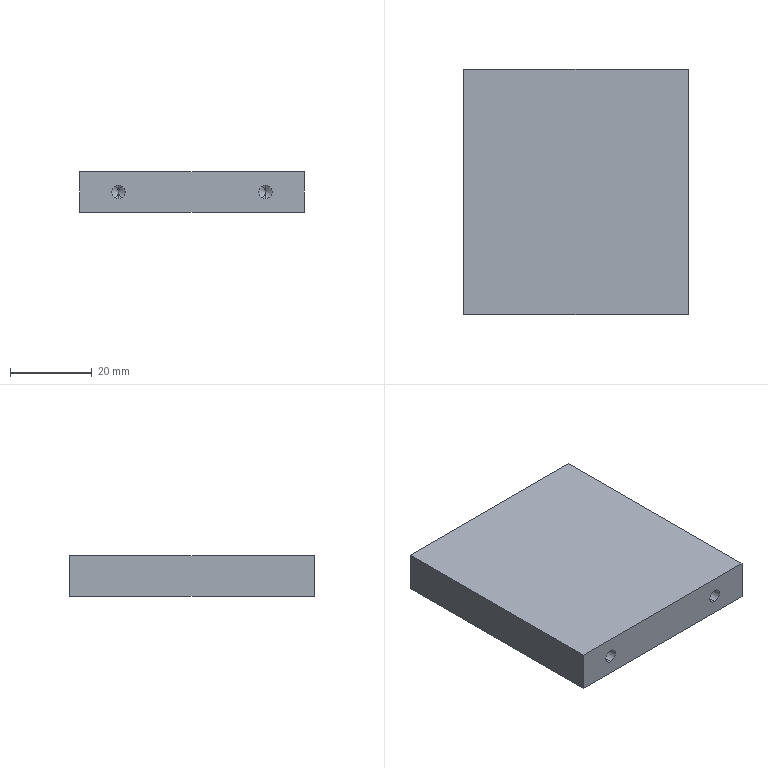Part | SolidWorks | features Extrusion 1, HoleWzd 1, MirrorPattern 1 | 1 solid | 22 faces | box 55 x 60 x 10 mm | volume 32595 mm3 | cylinder 8 | cone 8 | plane 6 | commonest cylinder face diameters 3.3 x8
STEP:
#1=CARTESIAN_POINT('',(18.,18.5,-1.65));
#2=VERTEX_POINT('',#1);
#3=CARTESIAN_POINT('',(18.,18.5,1.65));
#4=VERTEX_POINT('',#3);
#5=CARTESIAN_POINT('',(18.,18.5,0.));
#6=DIRECTION('',(0.,1.,0.));
#7=DIRECTION('',(0.,0.,1.));
#8=AXIS2_PLACEMENT_3D('',#5,#6,#7);
#9=CIRCLE('',#8,1.65);
#10=EDGE_CURVE('',#2,#4,#9,.T.);
#11=ORIENTED_EDGE('',*,*,#10,.F.);
#12=CARTESIAN_POINT('',(18.,30.,-1.65));
#13=VERTEX_POINT('',#12);
#14=CARTESIAN_POINT('',(18.,30.,-1.65));
#15=DIRECTION('',(0.,1.,0.));
#16=VECTOR('',#15,1000.);
#17=LINE('',#14,#16);
#18=EDGE_CURVE('',#2,#13,#17,.T.);
#19=ORIENTED_EDGE('',*,*,#18,.T.);
#20=CARTESIAN_POINT('',(18.,30.,1.65));
#21=VERTEX_POINT('',#20);
#22=CARTESIAN_POINT('',(18.,30.,0.));
#23=DIRECTION('',(0.,1.,0.));
#24=DIRECTION('',(0.,0.,1.));
#25=AXIS2_PLACEMENT_3D('',#22,#23,#24);
#26=CIRCLE('',#25,1.65);
#27=EDGE_CURVE('',#13,#21,#26,.T.);
#28=ORIENTED_EDGE('',*,*,#27,.T.);
#29=CARTESIAN_POINT('',(18.,30.,1.65));
#30=DIRECTION('',(0.,1.,0.));
#31=VECTOR('',#30,1000.);
#32=LINE('',#29,#31);
#33=EDGE_CURVE('',#4,#21,#32,.T.);
#34=ORIENTED_EDGE('',*,*,#33,.F.);
#35=EDGE_LOOP('',(#11,#19,#28,#34));
#36=FACE_OUTER_BOUND('',#35,.T.);
#37=CARTESIAN_POINT('',(18.,30.,0.));
#38=DIRECTION('',(0.,1.,0.));
#39=DIRECTION('',(0.,0.,1.));
#40=AXIS2_PLACEMENT_3D('',#37,#38,#39);
#41=CYLINDRICAL_SURFACE('',#40,1.65);
#42=ADVANCED_FACE('',(#36),#41,.F.);
#43=CARTESIAN_POINT('',(18.,17.509,0.));
#44=VERTEX_POINT('',#43);
#45=CARTESIAN_POINT('',(18.,18.5,1.65));
#46=DIRECTION('',(0.,0.515,0.8572));
#47=VECTOR('',#46,1000.);
#48=LINE('',#45,#47);
#49=EDGE_CURVE('',#44,#4,#48,.T.);
#50=ORIENTED_EDGE('',*,*,#49,.F.);
#51=CARTESIAN_POINT('',(18.,18.5,-1.65));
#52=DIRECTION('',(0.,0.515,-0.8572));
#53=VECTOR('',#52,1000.);
#54=LINE('',#51,#53);
#55=EDGE_CURVE('',#44,#2,#54,.T.);
#56=ORIENTED_EDGE('',*,*,#55,.T.);
#57=ORIENTED_EDGE('',*,*,#10,.T.);
#58=EDGE_LOOP('',(#50,#56,#57));
#59=FACE_OUTER_BOUND('',#58,.T.);
#60=CARTESIAN_POINT('',(18.,18.5,0.));
#61=DIRECTION('',(0.,1.,0.));
#62=DIRECTION('',(0.,0.,1.));
#63=AXIS2_PLACEMENT_3D('',#60,#61,#62);
#64=CONICAL_SURFACE('',#63,1.65,1.03);
#65=ADVANCED_FACE('',(#59),#64,.F.);
#66=CARTESIAN_POINT('',(-18.,18.5,-1.65));
#67=VERTEX_POINT('',#66);
#68=CARTESIAN_POINT('',(-18.,18.5,1.65));
#69=VERTEX_POINT('',#68);
#70=CARTESIAN_POINT('',(-18.,18.5,0.));
#71=DIRECTION('',(0.,1.,0.));
#72=DIRECTION('',(0.,0.,1.));
#73=AXIS2_PLACEMENT_3D('',#70,#71,#72);
#74=CIRCLE('',#73,1.65);
#75=EDGE_CURVE('',#67,#69,#74,.T.);
#76=ORIENTED_EDGE('',*,*,#75,.F.);
#77=CARTESIAN_POINT('',(-18.,30.,-1.65));
#78=VERTEX_POINT('',#77);
#79=CARTESIAN_POINT('',(-18.,30.,-1.65));
#80=DIRECTION('',(0.,1.,0.));
#81=VECTOR('',#80,1000.);
#82=LINE('',#79,#81);
#83=EDGE_CURVE('',#67,#78,#82,.T.);
#84=ORIENTED_EDGE('',*,*,#83,.T.);
#85=CARTESIAN_POINT('',(-18.,30.,1.65));
#86=VERTEX_POINT('',#85);
#87=CARTESIAN_POINT('',(-18.,30.,0.));
#88=DIRECTION('',(0.,1.,0.));
#89=DIRECTION('',(0.,0.,1.));
#90=AXIS2_PLACEMENT_3D('',#87,#88,#89);
#91=CIRCLE('',#90,1.65);
#92=EDGE_CURVE('',#78,#86,#91,.T.);
#93=ORIENTED_EDGE('',*,*,#92,.T.);
#94=CARTESIAN_POINT('',(-18.,30.,1.65));
#95=DIRECTION('',(0.,1.,0.));
#96=VECTOR('',#95,1000.);
#97=LINE('',#94,#96);
#98=EDGE_CURVE('',#69,#86,#97,.T.);
#99=ORIENTED_EDGE('',*,*,#98,.F.);
#100=EDGE_LOOP('',(#76,#84,#93,#99));
#101=FACE_OUTER_BOUND('',#100,.T.);
#102=CARTESIAN_POINT('',(-18.,30.,0.));
#103=DIRECTION('',(0.,1.,0.));
#104=DIRECTION('',(0.,0.,1.));
#105=AXIS2_PLACEMENT_3D('',#102,#103,#104);
#106=CYLINDRICAL_SURFACE('',#105,1.65);
#107=ADVANCED_FACE('',(#101),#106,.F.);
#108=CARTESIAN_POINT('',(-18.,17.509,0.));
#109=VERTEX_POINT('',#108);
#110=CARTESIAN_POINT('',(-18.,18.5,1.65));
#111=DIRECTION('',(0.,0.515,0.8572));
#112=VECTOR('',#111,1000.);
#113=LINE('',#110,#112);
#114=EDGE_CURVE('',#109,#69,#113,.T.);
#115=ORIENTED_EDGE('',*,*,#114,.F.);
#116=CARTESIAN_POINT('',(-18.,18.5,-1.65));
#117=DIRECTION('',(0.,0.515,-0.8572));
#118=VECTOR('',#117,1000.);
#119=LINE('',#116,#118);
#120=EDGE_CURVE('',#109,#67,#119,.T.);
#121=ORIENTED_EDGE('',*,*,#120,.T.);
#122=ORIENTED_EDGE('',*,*,#75,.T.);
#123=EDGE_LOOP('',(#115,#121,#122));
#124=FACE_OUTER_BOUND('',#123,.T.);
#125=CARTESIAN_POINT('',(-18.,18.5,0.));
#126=DIRECTION('',(0.,1.,0.));
#127=DIRECTION('',(0.,0.,1.));
#128=AXIS2_PLACEMENT_3D('',#125,#126,#127);
#129=CONICAL_SURFACE('',#128,1.65,1.03);
#130=ADVANCED_FACE('',(#124),#129,.F.);
#131=CARTESIAN_POINT('',(18.,-18.5,1.65));
#132=VERTEX_POINT('',#131);
#133=CARTESIAN_POINT('',(18.,-18.5,-1.65));
#134=VERTEX_POINT('',#133);
#135=CARTESIAN_POINT('',(18.,-18.5,0.));
#136=DIRECTION('',(0.,-1.,0.));
#137=DIRECTION('',(0.,0.,-1.));
#138=AXIS2_PLACEMENT_3D('',#135,#136,#137);
#139=CIRCLE('',#138,1.65);
#140=EDGE_CURVE('',#132,#134,#139,.T.);
#141=ORIENTED_EDGE('',*,*,#140,.F.);
#142=CARTESIAN_POINT('',(18.,-30.,1.65));
#143=VERTEX_POINT('',#142);
#144=CARTESIAN_POINT('',(18.,-30.,1.65));
#145=DIRECTION('',(0.,-1.,0.));
#146=VECTOR('',#145,1000.);
#147=LINE('',#144,#146);
#148=EDGE_CURVE('',#132,#143,#147,.T.);
#149=ORIENTED_EDGE('',*,*,#148,.T.);
#150=CARTESIAN_POINT('',(18.,-30.,-1.65));
#151=VERTEX_POINT('',#150);
#152=CARTESIAN_POINT('',(18.,-30.,0.));
#153=DIRECTION('',(0.,-1.,0.));
#154=DIRECTION('',(0.,0.,-1.));
#155=AXIS2_PLACEMENT_3D('',#152,#153,#154);
#156=CIRCLE('',#155,1.65);
#157=EDGE_CURVE('',#143,#151,#156,.T.);
#158=ORIENTED_EDGE('',*,*,#157,.T.);
#159=CARTESIAN_POINT('',(18.,-30.,-1.65));
#160=DIRECTION('',(0.,-1.,0.));
#161=VECTOR('',#160,1000.);
#162=LINE('',#159,#161);
#163=EDGE_CURVE('',#134,#151,#162,.T.);
#164=ORIENTED_EDGE('',*,*,#163,.F.);
#165=EDGE_LOOP('',(#141,#149,#158,#164));
#166=FACE_OUTER_BOUND('',#165,.T.);
#167=CARTESIAN_POINT('',(18.,-30.,0.));
#168=DIRECTION('',(0.,-1.,0.));
#169=DIRECTION('',(0.,0.,-1.));
#170=AXIS2_PLACEMENT_3D('',#167,#168,#169);
#171=CYLINDRICAL_SURFACE('',#170,1.65);
#172=ADVANCED_FACE('',(#166),#171,.F.);
#173=CARTESIAN_POINT('',(18.,-17.509,0.));
#174=VERTEX_POINT('',#173);
#175=CARTESIAN_POINT('',(18.,-18.5,-1.65));
#176=DIRECTION('',(0.,-0.515,-0.8572));
#177=VECTOR('',#176,1000.);
#178=LINE('',#175,#177);
#179=EDGE_CURVE('',#174,#134,#178,.T.);
#180=ORIENTED_EDGE('',*,*,#179,.F.);
#181=CARTESIAN_POINT('',(18.,-18.5,1.65));
#182=DIRECTION('',(0.,-0.515,0.8572));
#183=VECTOR('',#182,1000.);
#184=LINE('',#181,#183);
#185=EDGE_CURVE('',#174,#132,#184,.T.);
#186=ORIENTED_EDGE('',*,*,#185,.T.);
#187=ORIENTED_EDGE('',*,*,#140,.T.);
#188=EDGE_LOOP('',(#180,#186,#187));
#189=FACE_OUTER_BOUND('',#188,.T.);
#190=CARTESIAN_POINT('',(18.,-18.5,0.));
#191=DIRECTION('',(0.,-1.,0.));
#192=DIRECTION('',(0.,0.,-1.));
#193=AXIS2_PLACEMENT_3D('',#190,#191,#192);
#194=CONICAL_SURFACE('',#193,1.65,1.03);
#195=ADVANCED_FACE('',(#189),#194,.F.);
#196=CARTESIAN_POINT('',(-18.,-18.5,1.65));
#197=VERTEX_POINT('',#196);
#198=CARTESIAN_POINT('',(-18.,-18.5,-1.65));
#199=VERTEX_POINT('',#198);
#200=CARTESIAN_POINT('',(-18.,-18.5,0.));
#201=DIRECTION('',(0.,-1.,0.));
#202=DIRECTION('',(0.,0.,-1.));
#203=AXIS2_PLACEMENT_3D('',#200,#201,#202);
#204=CIRCLE('',#203,1.65);
#205=EDGE_CURVE('',#197,#199,#204,.T.);
#206=ORIENTED_EDGE('',*,*,#205,.F.);
#207=CARTESIAN_POINT('',(-18.,-30.,1.65));
#208=VERTEX_POINT('',#207);
#209=CARTESIAN_POINT('',(-18.,-30.,1.65));
#210=DIRECTION('',(0.,-1.,0.));
#211=VECTOR('',#210,1000.);
#212=LINE('',#209,#211);
#213=EDGE_CURVE('',#197,#208,#212,.T.);
#214=ORIENTED_EDGE('',*,*,#213,.T.);
#215=CARTESIAN_POINT('',(-18.,-30.,-1.65));
#216=VERTEX_POINT('',#215);
#217=CARTESIAN_POINT('',(-18.,-30.,0.));
#218=DIRECTION('',(0.,-1.,0.));
#219=DIRECTION('',(0.,0.,-1.));
#220=AXIS2_PLACEMENT_3D('',#217,#218,#219);
#221=CIRCLE('',#220,1.65);
#222=EDGE_CURVE('',#208,#216,#221,.T.);
#223=ORIENTED_EDGE('',*,*,#222,.T.);
#224=CARTESIAN_POINT('',(-18.,-30.,-1.65));
#225=DIRECTION('',(0.,-1.,0.));
#226=VECTOR('',#225,1000.);
#227=LINE('',#224,#226);
#228=EDGE_CURVE('',#199,#216,#227,.T.);
#229=ORIENTED_EDGE('',*,*,#228,.F.);
#230=EDGE_LOOP('',(#206,#214,#223,#229));
#231=FACE_OUTER_BOUND('',#230,.T.);
#232=CARTESIAN_POINT('',(-18.,-30.,0.));
#233=DIRECTION('',(0.,-1.,0.));
#234=DIRECTION('',(0.,0.,-1.));
#235=AXIS2_PLACEMENT_3D('',#232,#233,#234);
#236=CYLINDRICAL_SURFACE('',#235,1.65);
#237=ADVANCED_FACE('',(#231),#236,.F.);
#238=CARTESIAN_POINT('',(-18.,-17.509,0.));
#239=VERTEX_POINT('',#238);
#240=CARTESIAN_POINT('',(-18.,-18.5,-1.65));
#241=DIRECTION('',(0.,-0.515,-0.8572));
#242=VECTOR('',#241,1000.);
#243=LINE('',#240,#242);
#244=EDGE_CURVE('',#239,#199,#243,.T.);
#245=ORIENTED_EDGE('',*,*,#244,.F.);
#246=CARTESIAN_POINT('',(-18.,-18.5,1.65));
#247=DIRECTION('',(0.,-0.515,0.8572));
#248=VECTOR('',#247,1000.);
#249=LINE('',#246,#248);
#250=EDGE_CURVE('',#239,#197,#249,.T.);
#251=ORIENTED_EDGE('',*,*,#250,.T.);
#252=ORIENTED_EDGE('',*,*,#205,.T.);
#253=EDGE_LOOP('',(#245,#251,#252));
#254=FACE_OUTER_BOUND('',#253,.T.);
#255=CARTESIAN_POINT('',(-18.,-18.5,0.));
#256=DIRECTION('',(0.,-1.,0.));
#257=DIRECTION('',(0.,0.,-1.));
#258=AXIS2_PLACEMENT_3D('',#255,#256,#257);
#259=CONICAL_SURFACE('',#258,1.65,1.03);
#260=ADVANCED_FACE('',(#254),#259,.F.);
#261=CARTESIAN_POINT('',(27.5,-30.,-5.));
#262=VERTEX_POINT('',#261);
#263=CARTESIAN_POINT('',(27.5,30.,-5.));
#264=VERTEX_POINT('',#263);
#265=CARTESIAN_POINT('',(27.5,30.,-5.));
#266=DIRECTION('',(0.,1.,0.));
#267=VECTOR('',#266,1000.);
#268=LINE('',#265,#267);
#269=EDGE_CURVE('',#262,#264,#268,.T.);
#270=ORIENTED_EDGE('',*,*,#269,.T.);
#271=CARTESIAN_POINT('',(27.5,30.,5.));
#272=VERTEX_POINT('',#271);
#273=CARTESIAN_POINT('',(27.5,30.,5.));
#274=DIRECTION('',(0.,0.,-1.));
#275=VECTOR('',#274,1000.);
#276=LINE('',#273,#275);
#277=EDGE_CURVE('',#272,#264,#276,.T.);
#278=ORIENTED_EDGE('',*,*,#277,.F.);
#279=CARTESIAN_POINT('',(27.5,-30.,5.));
#280=VERTEX_POINT('',#279);
#281=CARTESIAN_POINT('',(27.5,30.,5.));
#282=DIRECTION('',(0.,1.,0.));
#283=VECTOR('',#282,1000.);
#284=LINE('',#281,#283);
#285=EDGE_CURVE('',#280,#272,#284,.T.);
#286=ORIENTED_EDGE('',*,*,#285,.F.);
#287=CARTESIAN_POINT('',(27.5,-30.,5.));
#288=DIRECTION('',(0.,0.,-1.));
#289=VECTOR('',#288,1000.);
#290=LINE('',#287,#289);
#291=EDGE_CURVE('',#280,#262,#290,.T.);
#292=ORIENTED_EDGE('',*,*,#291,.T.);
#293=EDGE_LOOP('',(#270,#278,#286,#292));
#294=FACE_OUTER_BOUND('',#293,.T.);
#295=CARTESIAN_POINT('',(27.5,30.,5.));
#296=DIRECTION('',(-1.,0.,0.));
#297=DIRECTION('',(0.,-1.,0.));
#298=AXIS2_PLACEMENT_3D('',#295,#296,#297);
#299=PLANE('',#298);
#300=ADVANCED_FACE('',(#294),#299,.F.);
#301=CARTESIAN_POINT('',(18.,30.,0.));
#302=DIRECTION('',(0.,1.,0.));
#303=DIRECTION('',(0.,0.,1.));
#304=AXIS2_PLACEMENT_3D('',#301,#302,#303);
#305=CIRCLE('',#304,1.65);
#306=EDGE_CURVE('',#21,#13,#305,.T.);
#307=ORIENTED_EDGE('',*,*,#306,.F.);
#308=ORIENTED_EDGE('',*,*,#27,.F.);
#309=EDGE_LOOP('',(#307,#308));
#310=FACE_BOUND('',#309,.T.);
#311=CARTESIAN_POINT('',(-18.,30.,0.));
#312=DIRECTION('',(0.,1.,0.));
#313=DIRECTION('',(0.,0.,1.));
#314=AXIS2_PLACEMENT_3D('',#311,#312,#313);
#315=CIRCLE('',#314,1.65);
#316=EDGE_CURVE('',#86,#78,#315,.T.);
#317=ORIENTED_EDGE('',*,*,#316,.F.);
#318=ORIENTED_EDGE('',*,*,#92,.F.);
#319=EDGE_LOOP('',(#317,#318));
#320=FACE_BOUND('',#319,.T.);
#321=CARTESIAN_POINT('',(-27.5,30.,-5.));
#322=VERTEX_POINT('',#321);
#323=CARTESIAN_POINT('',(-27.5,30.,-5.));
#324=DIRECTION('',(-1.,0.,0.));
#325=VECTOR('',#324,1000.);
#326=LINE('',#323,#325);
#327=EDGE_CURVE('',#264,#322,#326,.T.);
#328=ORIENTED_EDGE('',*,*,#327,.T.);
#329=CARTESIAN_POINT('',(-27.5,30.,5.));
#330=VERTEX_POINT('',#329);
#331=CARTESIAN_POINT('',(-27.5,30.,5.));
#332=DIRECTION('',(0.,0.,-1.));
#333=VECTOR('',#332,1000.);
#334=LINE('',#331,#333);
#335=EDGE_CURVE('',#330,#322,#334,.T.);
#336=ORIENTED_EDGE('',*,*,#335,.F.);
#337=CARTESIAN_POINT('',(-27.5,30.,5.));
#338=DIRECTION('',(-1.,0.,0.));
#339=VECTOR('',#338,1000.);
#340=LINE('',#337,#339);
#341=EDGE_CURVE('',#272,#330,#340,.T.);
#342=ORIENTED_EDGE('',*,*,#341,.F.);
#343=ORIENTED_EDGE('',*,*,#277,.T.);
#344=EDGE_LOOP('',(#328,#336,#342,#343));
#345=FACE_OUTER_BOUND('',#344,.T.);
#346=CARTESIAN_POINT('',(-27.5,30.,5.));
#347=DIRECTION('',(0.,-1.,0.));
#348=DIRECTION('',(0.,0.,-1.));
#349=AXIS2_PLACEMENT_3D('',#346,#347,#348);
#350=PLANE('',#349);
#351=ADVANCED_FACE('',(#310,#320,#345),#350,.F.);
#352=CARTESIAN_POINT('',(-27.5,-30.,-5.));
#353=VERTEX_POINT('',#352);
#354=CARTESIAN_POINT('',(-27.5,30.,-5.));
#355=DIRECTION('',(0.,-1.,0.));
#356=VECTOR('',#355,1000.);
#357=LINE('',#354,#356);
#358=EDGE_CURVE('',#322,#353,#357,.T.);
#359=ORIENTED_EDGE('',*,*,#358,.T.);
#360=CARTESIAN_POINT('',(-27.5,-30.,5.));
#361=VERTEX_POINT('',#360);
#362=CARTESIAN_POINT('',(-27.5,-30.,5.));
#363=DIRECTION('',(0.,0.,-1.));
#364=VECTOR('',#363,1000.);
#365=LINE('',#362,#364);
#366=EDGE_CURVE('',#361,#353,#365,.T.);
#367=ORIENTED_EDGE('',*,*,#366,.F.);
#368=CARTESIAN_POINT('',(-27.5,30.,5.));
#369=DIRECTION('',(0.,-1.,0.));
#370=VECTOR('',#369,1000.);
#371=LINE('',#368,#370);
#372=EDGE_CURVE('',#330,#361,#371,.T.);
#373=ORIENTED_EDGE('',*,*,#372,.F.);
#374=ORIENTED_EDGE('',*,*,#335,.T.);
#375=EDGE_LOOP('',(#359,#367,#373,#374));
#376=FACE_OUTER_BOUND('',#375,.T.);
#377=CARTESIAN_POINT('',(-27.5,30.,5.));
#378=DIRECTION('',(1.,0.,0.));
#379=DIRECTION('',(0.,1.,0.));
#380=AXIS2_PLACEMENT_3D('',#377,#378,#379);
#381=PLANE('',#380);
#382=ADVANCED_FACE('',(#376),#381,.F.);
#383=CARTESIAN_POINT('',(18.,-30.,0.));
#384=DIRECTION('',(0.,-1.,0.));
#385=DIRECTION('',(0.,0.,-1.));
#386=AXIS2_PLACEMENT_3D('',#383,#384,#385);
#387=CIRCLE('',#386,1.65);
#388=EDGE_CURVE('',#151,#143,#387,.T.);
#389=ORIENTED_EDGE('',*,*,#388,.F.);
#390=ORIENTED_EDGE('',*,*,#157,.F.);
#391=EDGE_LOOP('',(#389,#390));
#392=FACE_BOUND('',#391,.T.);
#393=CARTESIAN_POINT('',(-18.,-30.,0.));
#394=DIRECTION('',(0.,-1.,0.));
#395=DIRECTION('',(0.,0.,-1.));
#396=AXIS2_PLACEMENT_3D('',#393,#394,#395);
#397=CIRCLE('',#396,1.65);
#398=EDGE_CURVE('',#216,#208,#397,.T.);
#399=ORIENTED_EDGE('',*,*,#398,.F.);
#400=ORIENTED_EDGE('',*,*,#222,.F.);
#401=EDGE_LOOP('',(#399,#400));
#402=FACE_BOUND('',#401,.T.);
#403=CARTESIAN_POINT('',(-27.5,-30.,-5.));
#404=DIRECTION('',(1.,0.,0.));
#405=VECTOR('',#404,1000.);
#406=LINE('',#403,#405);
#407=EDGE_CURVE('',#353,#262,#406,.T.);
#408=ORIENTED_EDGE('',*,*,#407,.T.);
#409=ORIENTED_EDGE('',*,*,#291,.F.);
#410=CARTESIAN_POINT('',(-27.5,-30.,5.));
#411=DIRECTION('',(1.,0.,0.));
#412=VECTOR('',#411,1000.);
#413=LINE('',#410,#412);
#414=EDGE_CURVE('',#361,#280,#413,.T.);
#415=ORIENTED_EDGE('',*,*,#414,.F.);
#416=ORIENTED_EDGE('',*,*,#366,.T.);
#417=EDGE_LOOP('',(#408,#409,#415,#416));
#418=FACE_OUTER_BOUND('',#417,.T.);
#419=CARTESIAN_POINT('',(-27.5,-30.,5.));
#420=DIRECTION('',(0.,1.,0.));
#421=DIRECTION('',(0.,0.,1.));
#422=AXIS2_PLACEMENT_3D('',#419,#420,#421);
#423=PLANE('',#422);
#424=ADVANCED_FACE('',(#392,#402,#418),#423,.F.);
#425=ORIENTED_EDGE('',*,*,#285,.T.);
#426=ORIENTED_EDGE('',*,*,#341,.T.);
#427=ORIENTED_EDGE('',*,*,#372,.T.);
#428=ORIENTED_EDGE('',*,*,#414,.T.);
#429=EDGE_LOOP('',(#425,#426,#427,#428));
#430=FACE_OUTER_BOUND('',#429,.T.);
#431=CARTESIAN_POINT('',(0.,0.,5.));
#432=DIRECTION('',(0.,0.,1.));
#433=DIRECTION('',(1.,0.,0.));
#434=AXIS2_PLACEMENT_3D('',#431,#432,#433);
#435=PLANE('',#434);
#436=ADVANCED_FACE('',(#430),#435,.T.);
#437=ORIENTED_EDGE('',*,*,#269,.F.);
#438=ORIENTED_EDGE('',*,*,#407,.F.);
#439=ORIENTED_EDGE('',*,*,#358,.F.);
#440=ORIENTED_EDGE('',*,*,#327,.F.);
#441=EDGE_LOOP('',(#437,#438,#439,#440));
#442=FACE_OUTER_BOUND('',#441,.T.);
#443=CARTESIAN_POINT('',(0.,0.,-5.));
#444=DIRECTION('',(0.,0.,1.));
#445=DIRECTION('',(1.,0.,0.));
#446=AXIS2_PLACEMENT_3D('',#443,#444,#445);
#447=PLANE('',#446);
#448=ADVANCED_FACE('',(#442),#447,.F.);
#449=ORIENTED_EDGE('',*,*,#250,.F.);
#450=ORIENTED_EDGE('',*,*,#244,.T.);
#451=CARTESIAN_POINT('',(-18.,-18.5,0.));
#452=DIRECTION('',(0.,-1.,0.));
#453=DIRECTION('',(0.,0.,-1.));
#454=AXIS2_PLACEMENT_3D('',#451,#452,#453);
#455=CIRCLE('',#454,1.65);
#456=EDGE_CURVE('',#199,#197,#455,.T.);
#457=ORIENTED_EDGE('',*,*,#456,.T.);
#458=EDGE_LOOP('',(#449,#450,#457));
#459=FACE_OUTER_BOUND('',#458,.T.);
#460=CARTESIAN_POINT('',(-18.,-18.5,0.));
#461=DIRECTION('',(0.,-1.,0.));
#462=DIRECTION('',(0.,0.,-1.));
#463=AXIS2_PLACEMENT_3D('',#460,#461,#462);
#464=CONICAL_SURFACE('',#463,1.65,1.03);
#465=ADVANCED_FACE('',(#459),#464,.F.);
#466=ORIENTED_EDGE('',*,*,#213,.F.);
#467=ORIENTED_EDGE('',*,*,#456,.F.);
#468=ORIENTED_EDGE('',*,*,#228,.T.);
#469=ORIENTED_EDGE('',*,*,#398,.T.);
#470=EDGE_LOOP('',(#466,#467,#468,#469));
#471=FACE_OUTER_BOUND('',#470,.T.);
#472=CARTESIAN_POINT('',(-18.,-30.,0.));
#473=DIRECTION('',(0.,-1.,0.));
#474=DIRECTION('',(0.,0.,-1.));
#475=AXIS2_PLACEMENT_3D('',#472,#473,#474);
#476=CYLINDRICAL_SURFACE('',#475,1.65);
#477=ADVANCED_FACE('',(#471),#476,.F.);
#478=ORIENTED_EDGE('',*,*,#185,.F.);
#479=ORIENTED_EDGE('',*,*,#179,.T.);
#480=CARTESIAN_POINT('',(18.,-18.5,0.));
#481=DIRECTION('',(0.,-1.,0.));
#482=DIRECTION('',(0.,0.,-1.));
#483=AXIS2_PLACEMENT_3D('',#480,#481,#482);
#484=CIRCLE('',#483,1.65);
#485=EDGE_CURVE('',#134,#132,#484,.T.);
#486=ORIENTED_EDGE('',*,*,#485,.T.);
#487=EDGE_LOOP('',(#478,#479,#486));
#488=FACE_OUTER_BOUND('',#487,.T.);
#489=CARTESIAN_POINT('',(18.,-18.5,0.));
#490=DIRECTION('',(0.,-1.,0.));
#491=DIRECTION('',(0.,0.,-1.));
#492=AXIS2_PLACEMENT_3D('',#489,#490,#491);
#493=CONICAL_SURFACE('',#492,1.65,1.03);
#494=ADVANCED_FACE('',(#488),#493,.F.);
#495=ORIENTED_EDGE('',*,*,#148,.F.);
#496=ORIENTED_EDGE('',*,*,#485,.F.);
#497=ORIENTED_EDGE('',*,*,#163,.T.);
#498=ORIENTED_EDGE('',*,*,#388,.T.);
#499=EDGE_LOOP('',(#495,#496,#497,#498));
#500=FACE_OUTER_BOUND('',#499,.T.);
#501=CARTESIAN_POINT('',(18.,-30.,0.));
#502=DIRECTION('',(0.,-1.,0.));
#503=DIRECTION('',(0.,0.,-1.));
#504=AXIS2_PLACEMENT_3D('',#501,#502,#503);
#505=CYLINDRICAL_SURFACE('',#504,1.65);
#506=ADVANCED_FACE('',(#500),#505,.F.);
#507=ORIENTED_EDGE('',*,*,#120,.F.);
#508=ORIENTED_EDGE('',*,*,#114,.T.);
#509=CARTESIAN_POINT('',(-18.,18.5,0.));
#510=DIRECTION('',(0.,1.,0.));
#511=DIRECTION('',(0.,0.,1.));
#512=AXIS2_PLACEMENT_3D('',#509,#510,#511);
#513=CIRCLE('',#512,1.65);
#514=EDGE_CURVE('',#69,#67,#513,.T.);
#515=ORIENTED_EDGE('',*,*,#514,.T.);
#516=EDGE_LOOP('',(#507,#508,#515));
#517=FACE_OUTER_BOUND('',#516,.T.);
#518=CARTESIAN_POINT('',(-18.,18.5,0.));
#519=DIRECTION('',(0.,1.,0.));
#520=DIRECTION('',(0.,0.,1.));
#521=AXIS2_PLACEMENT_3D('',#518,#519,#520);
#522=CONICAL_SURFACE('',#521,1.65,1.03);
#523=ADVANCED_FACE('',(#517),#522,.F.);
#524=ORIENTED_EDGE('',*,*,#83,.F.);
#525=ORIENTED_EDGE('',*,*,#514,.F.);
#526=ORIENTED_EDGE('',*,*,#98,.T.);
#527=ORIENTED_EDGE('',*,*,#316,.T.);
#528=EDGE_LOOP('',(#524,#525,#526,#527));
#529=FACE_OUTER_BOUND('',#528,.T.);
#530=CARTESIAN_POINT('',(-18.,30.,0.));
#531=DIRECTION('',(0.,1.,0.));
#532=DIRECTION('',(0.,0.,1.));
#533=AXIS2_PLACEMENT_3D('',#530,#531,#532);
#534=CYLINDRICAL_SURFACE('',#533,1.65);
#535=ADVANCED_FACE('',(#529),#534,.F.);
#536=ORIENTED_EDGE('',*,*,#55,.F.);
#537=ORIENTED_EDGE('',*,*,#49,.T.);
#538=CARTESIAN_POINT('',(18.,18.5,0.));
#539=DIRECTION('',(0.,1.,0.));
#540=DIRECTION('',(0.,0.,1.));
#541=AXIS2_PLACEMENT_3D('',#538,#539,#540);
#542=CIRCLE('',#541,1.65);
#543=EDGE_CURVE('',#4,#2,#542,.T.);
#544=ORIENTED_EDGE('',*,*,#543,.T.);
#545=EDGE_LOOP('',(#536,#537,#544));
#546=FACE_OUTER_BOUND('',#545,.T.);
#547=CARTESIAN_POINT('',(18.,18.5,0.));
#548=DIRECTION('',(0.,1.,0.));
#549=DIRECTION('',(0.,0.,1.));
#550=AXIS2_PLACEMENT_3D('',#547,#548,#549);
#551=CONICAL_SURFACE('',#550,1.65,1.03);
#552=ADVANCED_FACE('',(#546),#551,.F.);
#553=ORIENTED_EDGE('',*,*,#18,.F.);
#554=ORIENTED_EDGE('',*,*,#543,.F.);
#555=ORIENTED_EDGE('',*,*,#33,.T.);
#556=ORIENTED_EDGE('',*,*,#306,.T.);
#557=EDGE_LOOP('',(#553,#554,#555,#556));
#558=FACE_OUTER_BOUND('',#557,.T.);
#559=CARTESIAN_POINT('',(18.,30.,0.));
#560=DIRECTION('',(0.,1.,0.));
#561=DIRECTION('',(0.,0.,1.));
#562=AXIS2_PLACEMENT_3D('',#559,#560,#561);
#563=CYLINDRICAL_SURFACE('',#562,1.65);
#564=ADVANCED_FACE('',(#558),#563,.F.);
#565=CLOSED_SHELL('',(#42,#65,#107,#130,#172,#195,#237,#260,#300,#351,#382,#424,#436,#448,#465,#477,#494,#506,#523,#535,#552,#564));
#566=MANIFOLD_SOLID_BREP('',#565);
#567=CARTESIAN_POINT('',(0.,0.,0.));
#568=DIRECTION('',(0.,0.,1.));
#569=DIRECTION('',(1.,0.,0.));
#570=AXIS2_PLACEMENT_3D('',#567,#568,#569);
#571=(LENGTH_UNIT()NAMED_UNIT(*)SI_UNIT(.MILLI.,.METRE.));
#572=UNCERTAINTY_MEASURE_WITH_UNIT(LENGTH_MEASURE(0.00001),#571,'','');
#573=(NAMED_UNIT(*)PLANE_ANGLE_UNIT()SI_UNIT($,.RADIAN.));
#574=(NAMED_UNIT(*)SI_UNIT($,.STERADIAN.)SOLID_ANGLE_UNIT());
#575=(GEOMETRIC_REPRESENTATION_CONTEXT(3)GLOBAL_UNCERTAINTY_ASSIGNED_CONTEXT((#572))GLOBAL_UNIT_ASSIGNED_CONTEXT((#571,#573,#574))REPRESENTATION_CONTEXT('',''));
#576=ADVANCED_BREP_SHAPE_REPRESENTATION('',(#566,#570),#575);